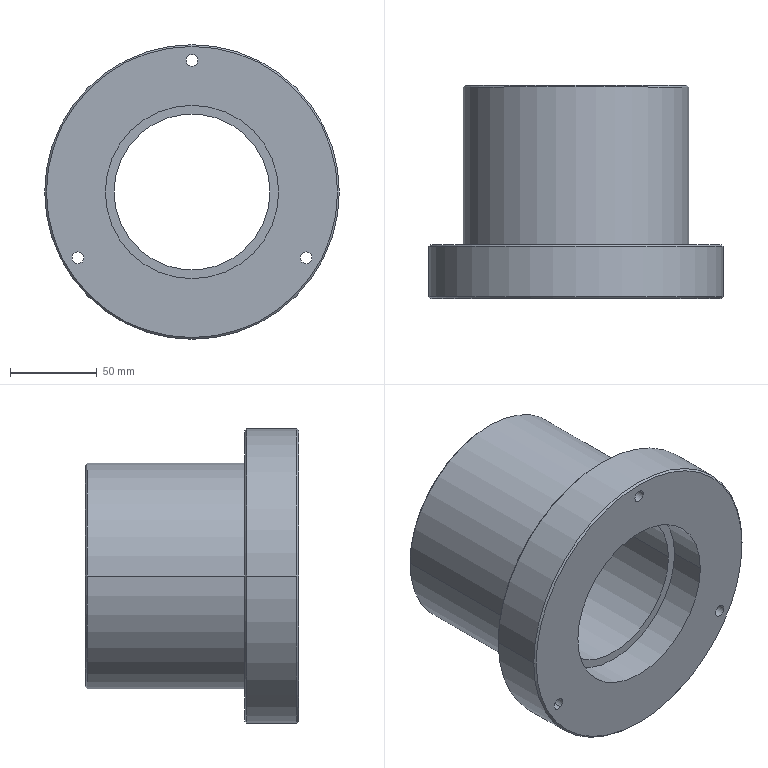Part | Creo | features CUT 9, CURVE 3, DATUM PLANE 3, PATTERN 2, CHAMFER 1, COORDINATE SYSTEM 1, PROTRUSION 1 | 1 solid | 45 faces | box 170 x 123 x 170 mm | volume 1070744 mm3 | cylinder 28 | plane 11 | cone 6 | commonest cylinder face diameters 5 x12 6.8 x6 100 x4 90 x2 130 x2 170 x2
STEP:
#1=CARTESIAN_POINT('',(0.,0.,0.));
#2=DIRECTION('',(0.,0.,1.));
#3=DIRECTION('',(1.,0.,0.));
#4=AXIS2_PLACEMENT_3D('',#1,#2,#3);
#5=CARTESIAN_POINT('',(50.,21.,0.));
#6=VERTEX_POINT('',#5);
#7=CARTESIAN_POINT('',(-50.,21.,0.));
#8=VERTEX_POINT('',#7);
#9=CARTESIAN_POINT('',(0.,21.,0.));
#10=DIRECTION('',(0.,-1.,0.));
#11=DIRECTION('',(1.,0.,0.));
#12=AXIS2_PLACEMENT_3D('',#9,#10,#11);
#13=CIRCLE('',#12,50.);
#14=EDGE_CURVE('',#6,#8,#13,.T.);
#15=ORIENTED_EDGE('',*,*,#14,.F.);
#16=CARTESIAN_POINT('',(0.,21.,0.));
#17=DIRECTION('',(0.,1.,0.));
#18=DIRECTION('',(1.,0.,0.));
#19=AXIS2_PLACEMENT_3D('',#16,#17,#18);
#20=CIRCLE('',#19,50.);
#21=EDGE_CURVE('',#6,#8,#20,.T.);
#22=ORIENTED_EDGE('',*,*,#21,.T.);
#23=EDGE_LOOP('',(#15,#22));
#24=FACE_OUTER_BOUND('',#23,.F.);
#25=CARTESIAN_POINT('',(45.,21.,0.));
#26=VERTEX_POINT('',#25);
#27=CARTESIAN_POINT('',(-45.,21.,0.));
#28=VERTEX_POINT('',#27);
#29=CARTESIAN_POINT('',(0.,21.,0.));
#30=DIRECTION('',(0.,1.,0.));
#31=DIRECTION('',(1.,0.,0.));
#32=AXIS2_PLACEMENT_3D('',#29,#30,#31);
#33=CIRCLE('',#32,45.);
#34=EDGE_CURVE('',#26,#28,#33,.T.);
#35=ORIENTED_EDGE('',*,*,#34,.F.);
#36=CARTESIAN_POINT('',(0.,21.,0.));
#37=DIRECTION('',(0.,-1.,0.));
#38=DIRECTION('',(1.,0.,0.));
#39=AXIS2_PLACEMENT_3D('',#36,#37,#38);
#40=CIRCLE('',#39,45.);
#41=EDGE_CURVE('',#26,#28,#40,.T.);
#42=ORIENTED_EDGE('',*,*,#41,.T.);
#43=EDGE_LOOP('',(#35,#42));
#44=FACE_BOUND('',#43,.F.);
#45=CARTESIAN_POINT('',(0.,21.,0.));
#46=DIRECTION('',(0.,1.,0.));
#47=DIRECTION('',(1.,0.,0.));
#48=AXIS2_PLACEMENT_3D('',#45,#46,#47);
#49=PLANE('',#48);
#50=ADVANCED_FACE('',(#24,#44),#49,.F.);
#51=CARTESIAN_POINT('',(45.,100.,0.));
#52=VERTEX_POINT('',#51);
#53=CARTESIAN_POINT('',(45.,100.,0.));
#54=DIRECTION('',(0.,-1.,0.));
#55=VECTOR('',#54,79.);
#56=LINE('',#53,#55);
#57=EDGE_CURVE('',#52,#26,#56,.T.);
#58=ORIENTED_EDGE('',*,*,#57,.T.);
#59=ORIENTED_EDGE('',*,*,#34,.T.);
#60=CARTESIAN_POINT('',(-45.,100.,0.));
#61=VERTEX_POINT('',#60);
#62=CARTESIAN_POINT('',(-45.,100.,0.));
#63=DIRECTION('',(0.,-1.,0.));
#64=VECTOR('',#63,79.);
#65=LINE('',#62,#64);
#66=EDGE_CURVE('',#61,#28,#65,.T.);
#67=ORIENTED_EDGE('',*,*,#66,.F.);
#68=CARTESIAN_POINT('',(0.,100.,0.));
#69=DIRECTION('',(0.,1.,0.));
#70=DIRECTION('',(1.,0.,0.));
#71=AXIS2_PLACEMENT_3D('',#68,#69,#70);
#72=CIRCLE('',#71,45.);
#73=EDGE_CURVE('',#52,#61,#72,.T.);
#74=ORIENTED_EDGE('',*,*,#73,.F.);
#75=EDGE_LOOP('',(#58,#59,#67,#74));
#76=FACE_OUTER_BOUND('',#75,.F.);
#77=CARTESIAN_POINT('',(0.,0.,0.));
#78=DIRECTION('',(0.,1.,0.));
#79=DIRECTION('',(1.,0.,0.));
#80=AXIS2_PLACEMENT_3D('',#77,#78,#79);
#81=CYLINDRICAL_SURFACE('',#80,45.);
#82=ADVANCED_FACE('',(#76),#81,.F.);
#83=ORIENTED_EDGE('',*,*,#57,.F.);
#84=CARTESIAN_POINT('',(0.,100.,0.));
#85=DIRECTION('',(0.,-1.,0.));
#86=DIRECTION('',(1.,0.,0.));
#87=AXIS2_PLACEMENT_3D('',#84,#85,#86);
#88=CIRCLE('',#87,45.);
#89=EDGE_CURVE('',#52,#61,#88,.T.);
#90=ORIENTED_EDGE('',*,*,#89,.T.);
#91=ORIENTED_EDGE('',*,*,#66,.T.);
#92=ORIENTED_EDGE('',*,*,#41,.F.);
#93=EDGE_LOOP('',(#83,#90,#91,#92));
#94=FACE_OUTER_BOUND('',#93,.F.);
#95=CARTESIAN_POINT('',(0.,0.,0.));
#96=DIRECTION('',(0.,1.,0.));
#97=DIRECTION('',(1.,0.,0.));
#98=AXIS2_PLACEMENT_3D('',#95,#96,#97);
#99=CYLINDRICAL_SURFACE('',#98,45.);
#100=ADVANCED_FACE('',(#94),#99,.F.);
#101=CARTESIAN_POINT('',(50.,100.,0.));
#102=VERTEX_POINT('',#101);
#103=CARTESIAN_POINT('',(-50.,100.,0.));
#104=VERTEX_POINT('',#103);
#105=CARTESIAN_POINT('',(0.,100.,0.));
#106=DIRECTION('',(0.,1.,0.));
#107=DIRECTION('',(1.,0.,0.));
#108=AXIS2_PLACEMENT_3D('',#105,#106,#107);
#109=CIRCLE('',#108,50.);
#110=EDGE_CURVE('',#102,#104,#109,.T.);
#111=ORIENTED_EDGE('',*,*,#110,.F.);
#112=CARTESIAN_POINT('',(0.,100.,0.));
#113=DIRECTION('',(0.,-1.,0.));
#114=DIRECTION('',(1.,0.,0.));
#115=AXIS2_PLACEMENT_3D('',#112,#113,#114);
#116=CIRCLE('',#115,50.);
#117=EDGE_CURVE('',#102,#104,#116,.T.);
#118=ORIENTED_EDGE('',*,*,#117,.T.);
#119=EDGE_LOOP('',(#111,#118));
#120=FACE_OUTER_BOUND('',#119,.F.);
#121=ORIENTED_EDGE('',*,*,#89,.F.);
#122=ORIENTED_EDGE('',*,*,#73,.T.);
#123=EDGE_LOOP('',(#121,#122));
#124=FACE_BOUND('',#123,.F.);
#125=CARTESIAN_POINT('',(0.,100.,0.));
#126=DIRECTION('',(0.,1.,0.));
#127=DIRECTION('',(1.,0.,0.));
#128=AXIS2_PLACEMENT_3D('',#125,#126,#127);
#129=PLANE('',#128);
#130=ADVANCED_FACE('',(#120,#124),#129,.T.);
#131=CARTESIAN_POINT('',(50.,123.,0.));
#132=VERTEX_POINT('',#131);
#133=CARTESIAN_POINT('',(50.,123.,0.));
#134=DIRECTION('',(0.,-1.,0.));
#135=VECTOR('',#134,23.);
#136=LINE('',#133,#135);
#137=EDGE_CURVE('',#132,#102,#136,.T.);
#138=ORIENTED_EDGE('',*,*,#137,.T.);
#139=ORIENTED_EDGE('',*,*,#110,.T.);
#140=CARTESIAN_POINT('',(-50.,123.,0.));
#141=VERTEX_POINT('',#140);
#142=CARTESIAN_POINT('',(-50.,123.,0.));
#143=DIRECTION('',(0.,-1.,0.));
#144=VECTOR('',#143,23.);
#145=LINE('',#142,#144);
#146=EDGE_CURVE('',#141,#104,#145,.T.);
#147=ORIENTED_EDGE('',*,*,#146,.F.);
#148=CARTESIAN_POINT('',(0.,123.,0.));
#149=DIRECTION('',(0.,1.,0.));
#150=DIRECTION('',(1.,0.,0.));
#151=AXIS2_PLACEMENT_3D('',#148,#149,#150);
#152=CIRCLE('',#151,50.);
#153=EDGE_CURVE('',#132,#141,#152,.T.);
#154=ORIENTED_EDGE('',*,*,#153,.F.);
#155=EDGE_LOOP('',(#138,#139,#147,#154));
#156=FACE_OUTER_BOUND('',#155,.F.);
#157=CARTESIAN_POINT('',(0.,0.,0.));
#158=DIRECTION('',(0.,1.,0.));
#159=DIRECTION('',(1.,0.,0.));
#160=AXIS2_PLACEMENT_3D('',#157,#158,#159);
#161=CYLINDRICAL_SURFACE('',#160,50.);
#162=ADVANCED_FACE('',(#156),#161,.F.);
#163=ORIENTED_EDGE('',*,*,#137,.F.);
#164=CARTESIAN_POINT('',(0.,123.,0.));
#165=DIRECTION('',(0.,-1.,0.));
#166=DIRECTION('',(1.,0.,0.));
#167=AXIS2_PLACEMENT_3D('',#164,#165,#166);
#168=CIRCLE('',#167,50.);
#169=EDGE_CURVE('',#132,#141,#168,.T.);
#170=ORIENTED_EDGE('',*,*,#169,.T.);
#171=ORIENTED_EDGE('',*,*,#146,.T.);
#172=ORIENTED_EDGE('',*,*,#117,.F.);
#173=EDGE_LOOP('',(#163,#170,#171,#172));
#174=FACE_OUTER_BOUND('',#173,.F.);
#175=CARTESIAN_POINT('',(0.,0.,0.));
#176=DIRECTION('',(0.,1.,0.));
#177=DIRECTION('',(1.,0.,0.));
#178=AXIS2_PLACEMENT_3D('',#175,#176,#177);
#179=CYLINDRICAL_SURFACE('',#178,50.);
#180=ADVANCED_FACE('',(#174),#179,.F.);
#181=CARTESIAN_POINT('',(64.,123.,0.));
#182=VERTEX_POINT('',#181);
#183=CARTESIAN_POINT('',(-64.,123.,0.));
#184=VERTEX_POINT('',#183);
#185=CARTESIAN_POINT('',(0.,123.,0.));
#186=DIRECTION('',(0.,1.,0.));
#187=DIRECTION('',(1.,0.,0.));
#188=AXIS2_PLACEMENT_3D('',#185,#186,#187);
#189=CIRCLE('',#188,64.);
#190=EDGE_CURVE('',#182,#184,#189,.T.);
#191=ORIENTED_EDGE('',*,*,#190,.F.);
#192=CARTESIAN_POINT('',(0.,123.,0.));
#193=DIRECTION('',(0.,1.,0.));
#194=DIRECTION('',(-1.,0.,0.));
#195=AXIS2_PLACEMENT_3D('',#192,#193,#194);
#196=CIRCLE('',#195,64.);
#197=EDGE_CURVE('',#184,#182,#196,.T.);
#198=ORIENTED_EDGE('',*,*,#197,.F.);
#199=EDGE_LOOP('',(#191,#198));
#200=FACE_OUTER_BOUND('',#199,.F.);
#201=ORIENTED_EDGE('',*,*,#169,.F.);
#202=ORIENTED_EDGE('',*,*,#153,.T.);
#203=EDGE_LOOP('',(#201,#202));
#204=FACE_BOUND('',#203,.F.);
#205=CARTESIAN_POINT('',(2.5,123.,-56.));
#206=VERTEX_POINT('',#205);
#207=CARTESIAN_POINT('',(-2.5,123.,-56.));
#208=VERTEX_POINT('',#207);
#209=CARTESIAN_POINT('',(0.,123.,-56.));
#210=DIRECTION('',(0.,1.,0.));
#211=DIRECTION('',(1.,0.,0.));
#212=AXIS2_PLACEMENT_3D('',#209,#210,#211);
#213=CIRCLE('',#212,2.5);
#214=EDGE_CURVE('',#206,#208,#213,.T.);
#215=ORIENTED_EDGE('',*,*,#214,.T.);
#216=CARTESIAN_POINT('',(0.,123.,-56.));
#217=DIRECTION('',(0.,1.,0.));
#218=DIRECTION('',(-1.,0.,0.));
#219=AXIS2_PLACEMENT_3D('',#216,#217,#218);
#220=CIRCLE('',#219,2.5);
#221=EDGE_CURVE('',#208,#206,#220,.T.);
#222=ORIENTED_EDGE('',*,*,#221,.T.);
#223=EDGE_LOOP('',(#215,#222));
#224=FACE_BOUND('',#223,.F.);
#225=CARTESIAN_POINT('',(-47.247,123.,-30.165));
#226=VERTEX_POINT('',#225);
#227=CARTESIAN_POINT('',(-49.747,123.,-25.835));
#228=VERTEX_POINT('',#227);
#229=CARTESIAN_POINT('',(-48.497,123.,-28.));
#230=DIRECTION('',(0.,1.,0.));
#231=DIRECTION('',(0.5,0.,-0.866));
#232=AXIS2_PLACEMENT_3D('',#229,#230,#231);
#233=CIRCLE('',#232,2.5);
#234=EDGE_CURVE('',#226,#228,#233,.T.);
#235=ORIENTED_EDGE('',*,*,#234,.T.);
#236=CARTESIAN_POINT('',(-48.497,123.,-28.));
#237=DIRECTION('',(0.,1.,0.));
#238=DIRECTION('',(-0.5,0.,0.866));
#239=AXIS2_PLACEMENT_3D('',#236,#237,#238);
#240=CIRCLE('',#239,2.5);
#241=EDGE_CURVE('',#228,#226,#240,.T.);
#242=ORIENTED_EDGE('',*,*,#241,.T.);
#243=EDGE_LOOP('',(#235,#242));
#244=FACE_BOUND('',#243,.F.);
#245=CARTESIAN_POINT('',(-49.747,123.,25.835));
#246=VERTEX_POINT('',#245);
#247=CARTESIAN_POINT('',(-47.247,123.,30.165));
#248=VERTEX_POINT('',#247);
#249=CARTESIAN_POINT('',(-48.497,123.,28.));
#250=DIRECTION('',(0.,1.,0.));
#251=DIRECTION('',(-0.5,0.,-0.866));
#252=AXIS2_PLACEMENT_3D('',#249,#250,#251);
#253=CIRCLE('',#252,2.5);
#254=EDGE_CURVE('',#246,#248,#253,.T.);
#255=ORIENTED_EDGE('',*,*,#254,.T.);
#256=CARTESIAN_POINT('',(-48.497,123.,28.));
#257=DIRECTION('',(0.,1.,0.));
#258=DIRECTION('',(0.5,0.,0.866));
#259=AXIS2_PLACEMENT_3D('',#256,#257,#258);
#260=CIRCLE('',#259,2.5);
#261=EDGE_CURVE('',#248,#246,#260,.T.);
#262=ORIENTED_EDGE('',*,*,#261,.T.);
#263=EDGE_LOOP('',(#255,#262));
#264=FACE_BOUND('',#263,.F.);
#265=CARTESIAN_POINT('',(-2.5,123.,56.));
#266=VERTEX_POINT('',#265);
#267=CARTESIAN_POINT('',(2.5,123.,56.));
#268=VERTEX_POINT('',#267);
#269=CARTESIAN_POINT('',(0.,123.,56.));
#270=DIRECTION('',(0.,1.,0.));
#271=DIRECTION('',(-1.,0.,0.));
#272=AXIS2_PLACEMENT_3D('',#269,#270,#271);
#273=CIRCLE('',#272,2.5);
#274=EDGE_CURVE('',#266,#268,#273,.T.);
#275=ORIENTED_EDGE('',*,*,#274,.T.);
#276=CARTESIAN_POINT('',(0.,123.,56.));
#277=DIRECTION('',(0.,1.,0.));
#278=DIRECTION('',(1.,0.,0.));
#279=AXIS2_PLACEMENT_3D('',#276,#277,#278);
#280=CIRCLE('',#279,2.5);
#281=EDGE_CURVE('',#268,#266,#280,.T.);
#282=ORIENTED_EDGE('',*,*,#281,.T.);
#283=EDGE_LOOP('',(#275,#282));
#284=FACE_BOUND('',#283,.F.);
#285=CARTESIAN_POINT('',(47.247,123.,30.165));
#286=VERTEX_POINT('',#285);
#287=CARTESIAN_POINT('',(49.747,123.,25.835));
#288=VERTEX_POINT('',#287);
#289=CARTESIAN_POINT('',(48.497,123.,28.));
#290=DIRECTION('',(0.,1.,0.));
#291=DIRECTION('',(-0.5,0.,0.866));
#292=AXIS2_PLACEMENT_3D('',#289,#290,#291);
#293=CIRCLE('',#292,2.5);
#294=EDGE_CURVE('',#286,#288,#293,.T.);
#295=ORIENTED_EDGE('',*,*,#294,.T.);
#296=CARTESIAN_POINT('',(48.497,123.,28.));
#297=DIRECTION('',(0.,1.,0.));
#298=DIRECTION('',(0.5,0.,-0.866));
#299=AXIS2_PLACEMENT_3D('',#296,#297,#298);
#300=CIRCLE('',#299,2.5);
#301=EDGE_CURVE('',#288,#286,#300,.T.);
#302=ORIENTED_EDGE('',*,*,#301,.T.);
#303=EDGE_LOOP('',(#295,#302));
#304=FACE_BOUND('',#303,.F.);
#305=CARTESIAN_POINT('',(49.747,123.,-25.835));
#306=VERTEX_POINT('',#305);
#307=CARTESIAN_POINT('',(47.247,123.,-30.165));
#308=VERTEX_POINT('',#307);
#309=CARTESIAN_POINT('',(48.497,123.,-28.));
#310=DIRECTION('',(0.,1.,0.));
#311=DIRECTION('',(0.5,0.,0.866));
#312=AXIS2_PLACEMENT_3D('',#309,#310,#311);
#313=CIRCLE('',#312,2.5);
#314=EDGE_CURVE('',#306,#308,#313,.T.);
#315=ORIENTED_EDGE('',*,*,#314,.T.);
#316=CARTESIAN_POINT('',(48.497,123.,-28.));
#317=DIRECTION('',(0.,1.,0.));
#318=DIRECTION('',(-0.5,0.,-0.866));
#319=AXIS2_PLACEMENT_3D('',#316,#317,#318);
#320=CIRCLE('',#319,2.5);
#321=EDGE_CURVE('',#308,#306,#320,.T.);
#322=ORIENTED_EDGE('',*,*,#321,.T.);
#323=EDGE_LOOP('',(#315,#322));
#324=FACE_BOUND('',#323,.F.);
#325=CARTESIAN_POINT('',(0.,123.,0.));
#326=DIRECTION('',(0.,1.,0.));
#327=DIRECTION('',(1.,0.,0.));
#328=AXIS2_PLACEMENT_3D('',#325,#326,#327);
#329=PLANE('',#328);
#330=ADVANCED_FACE('',(#200,#204,#224,#244,#264,#284,#304,#324),#329,.T.);
#331=ORIENTED_EDGE('',*,*,#190,.T.);
#332=CARTESIAN_POINT('',(-65.,122.,0.));
#333=VERTEX_POINT('',#332);
#334=CARTESIAN_POINT('',(-64.,123.,0.000000019));
#335=DIRECTION('',(-0.7071,-0.7071,-0.000000003));
#336=VECTOR('',#335,1.414);
#337=LINE('',#334,#336);
#338=EDGE_CURVE('',#184,#333,#337,.T.);
#339=ORIENTED_EDGE('',*,*,#338,.T.);
#340=CARTESIAN_POINT('',(65.,122.,0.));
#341=VERTEX_POINT('',#340);
#342=CARTESIAN_POINT('',(0.,122.,0.));
#343=DIRECTION('',(0.,1.,0.));
#344=DIRECTION('',(1.,0.,0.));
#345=AXIS2_PLACEMENT_3D('',#342,#343,#344);
#346=CIRCLE('',#345,65.);
#347=EDGE_CURVE('',#341,#333,#346,.T.);
#348=ORIENTED_EDGE('',*,*,#347,.F.);
#349=CARTESIAN_POINT('',(64.,123.,-0.000000019));
#350=DIRECTION('',(0.7071,-0.7071,0.000000003));
#351=VECTOR('',#350,1.414);
#352=LINE('',#349,#351);
#353=EDGE_CURVE('',#182,#341,#352,.T.);
#354=ORIENTED_EDGE('',*,*,#353,.F.);
#355=EDGE_LOOP('',(#331,#339,#348,#354));
#356=FACE_OUTER_BOUND('',#355,.F.);
#357=CARTESIAN_POINT('',(0.,122.5,0.));
#358=DIRECTION('',(0.,-1.,0.));
#359=DIRECTION('',(0.,0.,-1.));
#360=AXIS2_PLACEMENT_3D('',#357,#358,#359);
#361=CONICAL_SURFACE('',#360,64.5,45.);
#362=ADVANCED_FACE('',(#356),#361,.T.);
#363=ORIENTED_EDGE('',*,*,#197,.T.);
#364=ORIENTED_EDGE('',*,*,#353,.T.);
#365=CARTESIAN_POINT('',(0.,122.,0.));
#366=DIRECTION('',(0.,1.,0.));
#367=DIRECTION('',(-1.,0.,0.));
#368=AXIS2_PLACEMENT_3D('',#365,#366,#367);
#369=CIRCLE('',#368,65.);
#370=EDGE_CURVE('',#333,#341,#369,.T.);
#371=ORIENTED_EDGE('',*,*,#370,.F.);
#372=ORIENTED_EDGE('',*,*,#338,.F.);
#373=EDGE_LOOP('',(#363,#364,#371,#372));
#374=FACE_OUTER_BOUND('',#373,.F.);
#375=CARTESIAN_POINT('',(0.,122.5,0.));
#376=DIRECTION('',(0.,-1.,0.));
#377=DIRECTION('',(0.,0.,-1.));
#378=AXIS2_PLACEMENT_3D('',#375,#376,#377);
#379=CONICAL_SURFACE('',#378,64.5,45.);
#380=ADVANCED_FACE('',(#374),#379,.T.);
#381=ORIENTED_EDGE('',*,*,#370,.T.);
#382=CARTESIAN_POINT('',(65.,31.,0.));
#383=VERTEX_POINT('',#382);
#384=CARTESIAN_POINT('',(65.,31.,0.));
#385=DIRECTION('',(0.,1.,0.));
#386=VECTOR('',#385,91.);
#387=LINE('',#384,#386);
#388=EDGE_CURVE('',#383,#341,#387,.T.);
#389=ORIENTED_EDGE('',*,*,#388,.F.);
#390=CARTESIAN_POINT('',(-65.,31.,0.));
#391=VERTEX_POINT('',#390);
#392=CARTESIAN_POINT('',(0.,31.,0.));
#393=DIRECTION('',(0.,-1.,0.));
#394=DIRECTION('',(1.,0.,0.));
#395=AXIS2_PLACEMENT_3D('',#392,#393,#394);
#396=CIRCLE('',#395,65.);
#397=EDGE_CURVE('',#383,#391,#396,.T.);
#398=ORIENTED_EDGE('',*,*,#397,.T.);
#399=CARTESIAN_POINT('',(-65.,31.,0.));
#400=DIRECTION('',(0.,1.,0.));
#401=VECTOR('',#400,91.);
#402=LINE('',#399,#401);
#403=EDGE_CURVE('',#391,#333,#402,.T.);
#404=ORIENTED_EDGE('',*,*,#403,.T.);
#405=EDGE_LOOP('',(#381,#389,#398,#404));
#406=FACE_OUTER_BOUND('',#405,.F.);
#407=CARTESIAN_POINT('',(0.,0.,0.));
#408=DIRECTION('',(0.,1.,0.));
#409=DIRECTION('',(1.,0.,0.));
#410=AXIS2_PLACEMENT_3D('',#407,#408,#409);
#411=CYLINDRICAL_SURFACE('',#410,65.);
#412=ADVANCED_FACE('',(#406),#411,.T.);
#413=ORIENTED_EDGE('',*,*,#347,.T.);
#414=ORIENTED_EDGE('',*,*,#403,.F.);
#415=CARTESIAN_POINT('',(0.,31.,0.));
#416=DIRECTION('',(0.,1.,0.));
#417=DIRECTION('',(1.,0.,0.));
#418=AXIS2_PLACEMENT_3D('',#415,#416,#417);
#419=CIRCLE('',#418,65.);
#420=EDGE_CURVE('',#383,#391,#419,.T.);
#421=ORIENTED_EDGE('',*,*,#420,.F.);
#422=ORIENTED_EDGE('',*,*,#388,.T.);
#423=EDGE_LOOP('',(#413,#414,#421,#422));
#424=FACE_OUTER_BOUND('',#423,.F.);
#425=CARTESIAN_POINT('',(0.,0.,0.));
#426=DIRECTION('',(0.,1.,0.));
#427=DIRECTION('',(1.,0.,0.));
#428=AXIS2_PLACEMENT_3D('',#425,#426,#427);
#429=CYLINDRICAL_SURFACE('',#428,65.);
#430=ADVANCED_FACE('',(#424),#429,.T.);
#431=CARTESIAN_POINT('',(84.,31.,0.));
#432=VERTEX_POINT('',#431);
#433=CARTESIAN_POINT('',(-84.,31.,0.));
#434=VERTEX_POINT('',#433);
#435=CARTESIAN_POINT('',(0.,31.,0.));
#436=DIRECTION('',(0.,1.,0.));
#437=DIRECTION('',(1.,0.,0.));
#438=AXIS2_PLACEMENT_3D('',#435,#436,#437);
#439=CIRCLE('',#438,84.);
#440=EDGE_CURVE('',#432,#434,#439,.T.);
#441=ORIENTED_EDGE('',*,*,#440,.F.);
#442=CARTESIAN_POINT('',(0.,31.,0.));
#443=DIRECTION('',(0.,1.,0.));
#444=DIRECTION('',(-1.,0.,0.));
#445=AXIS2_PLACEMENT_3D('',#442,#443,#444);
#446=CIRCLE('',#445,84.);
#447=EDGE_CURVE('',#434,#432,#446,.T.);
#448=ORIENTED_EDGE('',*,*,#447,.F.);
#449=EDGE_LOOP('',(#441,#448));
#450=FACE_OUTER_BOUND('',#449,.F.);
#451=CARTESIAN_POINT('',(3.4,31.,76.));
#452=VERTEX_POINT('',#451);
#453=CARTESIAN_POINT('',(-3.4,31.,76.));
#454=VERTEX_POINT('',#453);
#455=CARTESIAN_POINT('',(0.,31.,76.));
#456=DIRECTION('',(0.,-1.,0.));
#457=DIRECTION('',(1.,0.,0.));
#458=AXIS2_PLACEMENT_3D('',#455,#456,#457);
#459=CIRCLE('',#458,3.4);
#460=EDGE_CURVE('',#452,#454,#459,.T.);
#461=ORIENTED_EDGE('',*,*,#460,.F.);
#462=CARTESIAN_POINT('',(0.,31.,76.));
#463=DIRECTION('',(0.,-1.,0.));
#464=DIRECTION('',(-1.,0.,0.));
#465=AXIS2_PLACEMENT_3D('',#462,#463,#464);
#466=CIRCLE('',#465,3.4);
#467=EDGE_CURVE('',#454,#452,#466,.T.);
#468=ORIENTED_EDGE('',*,*,#467,.F.);
#469=EDGE_LOOP('',(#461,#468));
#470=FACE_BOUND('',#469,.F.);
#471=CARTESIAN_POINT('',(64.118,31.,-40.944));
#472=VERTEX_POINT('',#471);
#473=CARTESIAN_POINT('',(67.518,31.,-35.056));
#474=VERTEX_POINT('',#473);
#475=CARTESIAN_POINT('',(65.818,31.,-38.));
#476=DIRECTION('',(0.,-1.,0.));
#477=DIRECTION('',(-0.5,0.,-0.866));
#478=AXIS2_PLACEMENT_3D('',#475,#476,#477);
#479=CIRCLE('',#478,3.4);
#480=EDGE_CURVE('',#472,#474,#479,.T.);
#481=ORIENTED_EDGE('',*,*,#480,.F.);
#482=CARTESIAN_POINT('',(65.818,31.,-38.));
#483=DIRECTION('',(0.,-1.,0.));
#484=DIRECTION('',(0.5,0.,0.866));
#485=AXIS2_PLACEMENT_3D('',#482,#483,#484);
#486=CIRCLE('',#485,3.4);
#487=EDGE_CURVE('',#474,#472,#486,.T.);
#488=ORIENTED_EDGE('',*,*,#487,.F.);
#489=EDGE_LOOP('',(#481,#488));
#490=FACE_BOUND('',#489,.F.);
#491=CARTESIAN_POINT('',(-67.518,31.,-35.056));
#492=VERTEX_POINT('',#491);
#493=CARTESIAN_POINT('',(-64.118,31.,-40.944));
#494=VERTEX_POINT('',#493);
#495=CARTESIAN_POINT('',(-65.818,31.,-38.));
#496=DIRECTION('',(0.,-1.,0.));
#497=DIRECTION('',(-0.5,0.,0.866));
#498=AXIS2_PLACEMENT_3D('',#495,#496,#497);
#499=CIRCLE('',#498,3.4);
#500=EDGE_CURVE('',#492,#494,#499,.T.);
#501=ORIENTED_EDGE('',*,*,#500,.F.);
#502=CARTESIAN_POINT('',(-65.818,31.,-38.));
#503=DIRECTION('',(0.,-1.,0.));
#504=DIRECTION('',(0.5,0.,-0.866));
#505=AXIS2_PLACEMENT_3D('',#502,#503,#504);
#506=CIRCLE('',#505,3.4);
#507=EDGE_CURVE('',#494,#492,#506,.T.);
#508=ORIENTED_EDGE('',*,*,#507,.F.);
#509=EDGE_LOOP('',(#501,#508));
#510=FACE_BOUND('',#509,.F.);
#511=ORIENTED_EDGE('',*,*,#397,.F.);
#512=ORIENTED_EDGE('',*,*,#420,.T.);
#513=EDGE_LOOP('',(#511,#512));
#514=FACE_BOUND('',#513,.F.);
#515=CARTESIAN_POINT('',(0.,31.,0.));
#516=DIRECTION('',(0.,1.,0.));
#517=DIRECTION('',(1.,0.,0.));
#518=AXIS2_PLACEMENT_3D('',#515,#516,#517);
#519=PLANE('',#518);
#520=ADVANCED_FACE('',(#450,#470,#490,#510,#514),#519,.T.);
#521=CARTESIAN_POINT('',(3.4,0.,76.));
#522=VERTEX_POINT('',#521);
#523=CARTESIAN_POINT('',(-3.4,0.,76.));
#524=VERTEX_POINT('',#523);
#525=CARTESIAN_POINT('',(0.,0.,76.));
#526=DIRECTION('',(0.,-1.,0.));
#527=DIRECTION('',(1.,0.,0.));
#528=AXIS2_PLACEMENT_3D('',#525,#526,#527);
#529=CIRCLE('',#528,3.4);
#530=EDGE_CURVE('',#522,#524,#529,.T.);
#531=ORIENTED_EDGE('',*,*,#530,.F.);
#532=CARTESIAN_POINT('',(3.4,0.,76.));
#533=DIRECTION('',(0.,1.,0.));
#534=VECTOR('',#533,31.);
#535=LINE('',#532,#534);
#536=EDGE_CURVE('',#522,#452,#535,.T.);
#537=ORIENTED_EDGE('',*,*,#536,.T.);
#538=ORIENTED_EDGE('',*,*,#460,.T.);
#539=CARTESIAN_POINT('',(-3.4,0.,76.));
#540=DIRECTION('',(0.,1.,0.));
#541=VECTOR('',#540,31.);
#542=LINE('',#539,#541);
#543=EDGE_CURVE('',#524,#454,#542,.T.);
#544=ORIENTED_EDGE('',*,*,#543,.F.);
#545=EDGE_LOOP('',(#531,#537,#538,#544));
#546=FACE_OUTER_BOUND('',#545,.F.);
#547=CARTESIAN_POINT('',(0.,0.,76.));
#548=DIRECTION('',(0.,-1.,0.));
#549=DIRECTION('',(1.,0.,0.));
#550=AXIS2_PLACEMENT_3D('',#547,#548,#549);
#551=CYLINDRICAL_SURFACE('',#550,3.4);
#552=ADVANCED_FACE('',(#546),#551,.F.);
#553=CARTESIAN_POINT('',(84.,0.,0.));
#554=VERTEX_POINT('',#553);
#555=CARTESIAN_POINT('',(-84.,0.,0.));
#556=VERTEX_POINT('',#555);
#557=CARTESIAN_POINT('',(0.,0.,0.));
#558=DIRECTION('',(0.,1.,0.));
#559=DIRECTION('',(1.,0.,0.));
#560=AXIS2_PLACEMENT_3D('',#557,#558,#559);
#561=CIRCLE('',#560,84.);
#562=EDGE_CURVE('',#554,#556,#561,.T.);
#563=ORIENTED_EDGE('',*,*,#562,.T.);
#564=CARTESIAN_POINT('',(0.,0.,0.));
#565=DIRECTION('',(0.,1.,0.));
#566=DIRECTION('',(-1.,0.,0.));
#567=AXIS2_PLACEMENT_3D('',#564,#565,#566);
#568=CIRCLE('',#567,84.);
#569=EDGE_CURVE('',#556,#554,#568,.T.);
#570=ORIENTED_EDGE('',*,*,#569,.T.);
#571=EDGE_LOOP('',(#563,#570));
#572=FACE_OUTER_BOUND('',#571,.F.);
#573=ORIENTED_EDGE('',*,*,#530,.T.);
#574=CARTESIAN_POINT('',(0.,0.,76.));
#575=DIRECTION('',(0.,-1.,0.));
#576=DIRECTION('',(-1.,0.,0.));
#577=AXIS2_PLACEMENT_3D('',#574,#575,#576);
#578=CIRCLE('',#577,3.4);
#579=EDGE_CURVE('',#524,#522,#578,.T.);
#580=ORIENTED_EDGE('',*,*,#579,.T.);
#581=EDGE_LOOP('',(#573,#580));
#582=FACE_BOUND('',#581,.F.);
#583=CARTESIAN_POINT('',(64.118,0.,-40.944));
#584=VERTEX_POINT('',#583);
#585=CARTESIAN_POINT('',(67.518,0.,-35.056));
#586=VERTEX_POINT('',#585);
#587=CARTESIAN_POINT('',(65.818,0.,-38.));
#588=DIRECTION('',(0.,-1.,0.));
#589=DIRECTION('',(-0.5,0.,-0.866));
#590=AXIS2_PLACEMENT_3D('',#587,#588,#589);
#591=CIRCLE('',#590,3.4);
#592=EDGE_CURVE('',#584,#586,#591,.T.);
#593=ORIENTED_EDGE('',*,*,#592,.T.);
#594=CARTESIAN_POINT('',(65.818,0.,-38.));
#595=DIRECTION('',(0.,-1.,0.));
#596=DIRECTION('',(0.5,0.,0.866));
#597=AXIS2_PLACEMENT_3D('',#594,#595,#596);
#598=CIRCLE('',#597,3.4);
#599=EDGE_CURVE('',#586,#584,#598,.T.);
#600=ORIENTED_EDGE('',*,*,#599,.T.);
#601=EDGE_LOOP('',(#593,#600));
#602=FACE_BOUND('',#601,.F.);
#603=CARTESIAN_POINT('',(-67.518,0.,-35.056));
#604=VERTEX_POINT('',#603);
#605=CARTESIAN_POINT('',(-64.118,0.,-40.944));
#606=VERTEX_POINT('',#605);
#607=CARTESIAN_POINT('',(-65.818,0.,-38.));
#608=DIRECTION('',(0.,-1.,0.));
#609=DIRECTION('',(-0.5,0.,0.866));
#610=AXIS2_PLACEMENT_3D('',#607,#608,#609);
#611=CIRCLE('',#610,3.4);
#612=EDGE_CURVE('',#604,#606,#611,.T.);
#613=ORIENTED_EDGE('',*,*,#612,.T.);
#614=CARTESIAN_POINT('',(-65.818,0.,-38.));
#615=DIRECTION('',(0.,-1.,0.));
#616=DIRECTION('',(0.5,0.,-0.866));
#617=AXIS2_PLACEMENT_3D('',#614,#615,#616);
#618=CIRCLE('',#617,3.4);
#619=EDGE_CURVE('',#606,#604,#618,.T.);
#620=ORIENTED_EDGE('',*,*,#619,.T.);
#621=EDGE_LOOP('',(#613,#620));
#622=FACE_BOUND('',#621,.F.);
#623=CARTESIAN_POINT('',(50.,0.,0.));
#624=VERTEX_POINT('',#623);
#625=CARTESIAN_POINT('',(-50.,0.,0.));
#626=VERTEX_POINT('',#625);
#627=CARTESIAN_POINT('',(0.,0.,0.));
#628=DIRECTION('',(0.,1.,0.));
#629=DIRECTION('',(1.,0.,0.));
#630=AXIS2_PLACEMENT_3D('',#627,#628,#629);
#631=CIRCLE('',#630,50.);
#632=EDGE_CURVE('',#624,#626,#631,.T.);
#633=ORIENTED_EDGE('',*,*,#632,.F.);
#634=CARTESIAN_POINT('',(0.,0.,0.));
#635=DIRECTION('',(0.,-1.,0.));
#636=DIRECTION('',(1.,0.,0.));
#637=AXIS2_PLACEMENT_3D('',#634,#635,#636);
#638=CIRCLE('',#637,50.);
#639=EDGE_CURVE('',#624,#626,#638,.T.);
#640=ORIENTED_EDGE('',*,*,#639,.T.);
#641=EDGE_LOOP('',(#633,#640));
#642=FACE_BOUND('',#641,.F.);
#643=CARTESIAN_POINT('',(0.,0.,0.));
#644=DIRECTION('',(0.,1.,0.));
#645=DIRECTION('',(1.,0.,0.));
#646=AXIS2_PLACEMENT_3D('',#643,#644,#645);
#647=PLANE('',#646);
#648=ADVANCED_FACE('',(#572,#582,#602,#622,#642),#647,.F.);
#649=CARTESIAN_POINT('',(50.,21.,0.));
#650=DIRECTION('',(0.,-1.,0.));
#651=VECTOR('',#650,21.);
#652=LINE('',#649,#651);
#653=EDGE_CURVE('',#6,#624,#652,.T.);
#654=ORIENTED_EDGE('',*,*,#653,.T.);
#655=ORIENTED_EDGE('',*,*,#632,.T.);
#656=CARTESIAN_POINT('',(-50.,21.,0.));
#657=DIRECTION('',(0.,-1.,0.));
#658=VECTOR('',#657,21.);
#659=LINE('',#656,#658);
#660=EDGE_CURVE('',#8,#626,#659,.T.);
#661=ORIENTED_EDGE('',*,*,#660,.F.);
#662=ORIENTED_EDGE('',*,*,#21,.F.);
#663=EDGE_LOOP('',(#654,#655,#661,#662));
#664=FACE_OUTER_BOUND('',#663,.F.);
#665=CARTESIAN_POINT('',(0.,0.,0.));
#666=DIRECTION('',(0.,1.,0.));
#667=DIRECTION('',(1.,0.,0.));
#668=AXIS2_PLACEMENT_3D('',#665,#666,#667);
#669=CYLINDRICAL_SURFACE('',#668,50.);
#670=ADVANCED_FACE('',(#664),#669,.F.);
#671=ORIENTED_EDGE('',*,*,#653,.F.);
#672=ORIENTED_EDGE('',*,*,#14,.T.);
#673=ORIENTED_EDGE('',*,*,#660,.T.);
#674=ORIENTED_EDGE('',*,*,#639,.F.);
#675=EDGE_LOOP('',(#671,#672,#673,#674));
#676=FACE_OUTER_BOUND('',#675,.F.);
#677=CARTESIAN_POINT('',(0.,0.,0.));
#678=DIRECTION('',(0.,1.,0.));
#679=DIRECTION('',(1.,0.,0.));
#680=AXIS2_PLACEMENT_3D('',#677,#678,#679);
#681=CYLINDRICAL_SURFACE('',#680,50.);
#682=ADVANCED_FACE('',(#676),#681,.F.);
#683=ORIENTED_EDGE('',*,*,#579,.F.);
#684=ORIENTED_EDGE('',*,*,#543,.T.);
#685=ORIENTED_EDGE('',*,*,#467,.T.);
#686=ORIENTED_EDGE('',*,*,#536,.F.);
#687=EDGE_LOOP('',(#683,#684,#685,#686));
#688=FACE_OUTER_BOUND('',#687,.F.);
#689=CARTESIAN_POINT('',(0.,0.,76.));
#690=DIRECTION('',(0.,-1.,0.));
#691=DIRECTION('',(1.,0.,0.));
#692=AXIS2_PLACEMENT_3D('',#689,#690,#691);
#693=CYLINDRICAL_SURFACE('',#692,3.4);
#694=ADVANCED_FACE('',(#688),#693,.F.);
#695=ORIENTED_EDGE('',*,*,#592,.F.);
#696=CARTESIAN_POINT('',(64.118,0.,-40.944));
#697=DIRECTION('',(0.,1.,0.));
#698=VECTOR('',#697,31.);
#699=LINE('',#696,#698);
#700=EDGE_CURVE('',#584,#472,#699,.T.);
#701=ORIENTED_EDGE('',*,*,#700,.T.);
#702=ORIENTED_EDGE('',*,*,#480,.T.);
#703=CARTESIAN_POINT('',(67.518,0.,-35.056));
#704=DIRECTION('',(0.,1.,0.));
#705=VECTOR('',#704,31.);
#706=LINE('',#703,#705);
#707=EDGE_CURVE('',#586,#474,#706,.T.);
#708=ORIENTED_EDGE('',*,*,#707,.F.);
#709=EDGE_LOOP('',(#695,#701,#702,#708));
#710=FACE_OUTER_BOUND('',#709,.F.);
#711=CARTESIAN_POINT('',(65.818,0.,-38.));
#712=DIRECTION('',(0.,-1.,0.));
#713=DIRECTION('',(-0.5,0.,-0.866));
#714=AXIS2_PLACEMENT_3D('',#711,#712,#713);
#715=CYLINDRICAL_SURFACE('',#714,3.4);
#716=ADVANCED_FACE('',(#710),#715,.F.);
#717=ORIENTED_EDGE('',*,*,#599,.F.);
#718=ORIENTED_EDGE('',*,*,#707,.T.);
#719=ORIENTED_EDGE('',*,*,#487,.T.);
#720=ORIENTED_EDGE('',*,*,#700,.F.);
#721=EDGE_LOOP('',(#717,#718,#719,#720));
#722=FACE_OUTER_BOUND('',#721,.F.);
#723=CARTESIAN_POINT('',(65.818,0.,-38.));
#724=DIRECTION('',(0.,-1.,0.));
#725=DIRECTION('',(-0.5,0.,-0.866));
#726=AXIS2_PLACEMENT_3D('',#723,#724,#725);
#727=CYLINDRICAL_SURFACE('',#726,3.4);
#728=ADVANCED_FACE('',(#722),#727,.F.);
#729=ORIENTED_EDGE('',*,*,#612,.F.);
#730=CARTESIAN_POINT('',(-67.518,0.,-35.056));
#731=DIRECTION('',(0.,1.,0.));
#732=VECTOR('',#731,31.);
#733=LINE('',#730,#732);
#734=EDGE_CURVE('',#604,#492,#733,.T.);
#735=ORIENTED_EDGE('',*,*,#734,.T.);
#736=ORIENTED_EDGE('',*,*,#500,.T.);
#737=CARTESIAN_POINT('',(-64.118,0.,-40.944));
#738=DIRECTION('',(0.,1.,0.));
#739=VECTOR('',#738,31.);
#740=LINE('',#737,#739);
#741=EDGE_CURVE('',#606,#494,#740,.T.);
#742=ORIENTED_EDGE('',*,*,#741,.F.);
#743=EDGE_LOOP('',(#729,#735,#736,#742));
#744=FACE_OUTER_BOUND('',#743,.F.);
#745=CARTESIAN_POINT('',(-65.818,0.,-38.));
#746=DIRECTION('',(0.,-1.,0.));
#747=DIRECTION('',(-0.5,0.,0.866));
#748=AXIS2_PLACEMENT_3D('',#745,#746,#747);
#749=CYLINDRICAL_SURFACE('',#748,3.4);
#750=ADVANCED_FACE('',(#744),#749,.F.);
#751=ORIENTED_EDGE('',*,*,#619,.F.);
#752=ORIENTED_EDGE('',*,*,#741,.T.);
#753=ORIENTED_EDGE('',*,*,#507,.T.);
#754=ORIENTED_EDGE('',*,*,#734,.F.);
#755=EDGE_LOOP('',(#751,#752,#753,#754));
#756=FACE_OUTER_BOUND('',#755,.F.);
#757=CARTESIAN_POINT('',(-65.818,0.,-38.));
#758=DIRECTION('',(0.,-1.,0.));
#759=DIRECTION('',(-0.5,0.,0.866));
#760=AXIS2_PLACEMENT_3D('',#757,#758,#759);
#761=CYLINDRICAL_SURFACE('',#760,3.4);
#762=ADVANCED_FACE('',(#756),#761,.F.);
#763=CARTESIAN_POINT('',(85.,1.,0.));
#764=VERTEX_POINT('',#763);
#765=CARTESIAN_POINT('',(-85.,1.,0.));
#766=VERTEX_POINT('',#765);
#767=CARTESIAN_POINT('',(0.,1.,0.));
#768=DIRECTION('',(0.,1.,0.));
#769=DIRECTION('',(1.,0.,0.));
#770=AXIS2_PLACEMENT_3D('',#767,#768,#769);
#771=CIRCLE('',#770,85.);
#772=EDGE_CURVE('',#764,#766,#771,.T.);
#773=ORIENTED_EDGE('',*,*,#772,.T.);
#774=CARTESIAN_POINT('',(-85.,1.,-0.000000002));
#775=DIRECTION('',(0.7071,-0.7071,-0.000000001));
#776=VECTOR('',#775,1.414);
#777=LINE('',#774,#776);
#778=EDGE_CURVE('',#766,#556,#777,.T.);
#779=ORIENTED_EDGE('',*,*,#778,.T.);
#780=ORIENTED_EDGE('',*,*,#562,.F.);
#781=CARTESIAN_POINT('',(85.,1.,0.000000002));
#782=DIRECTION('',(-0.7071,-0.7071,0.000000001));
#783=VECTOR('',#782,1.414);
#784=LINE('',#781,#783);
#785=EDGE_CURVE('',#764,#554,#784,.T.);
#786=ORIENTED_EDGE('',*,*,#785,.F.);
#787=EDGE_LOOP('',(#773,#779,#780,#786));
#788=FACE_OUTER_BOUND('',#787,.F.);
#789=CARTESIAN_POINT('',(0.,0.5,0.));
#790=DIRECTION('',(0.,1.,0.));
#791=DIRECTION('',(0.,0.,-1.));
#792=AXIS2_PLACEMENT_3D('',#789,#790,#791);
#793=CONICAL_SURFACE('',#792,84.5,45.);
#794=ADVANCED_FACE('',(#788),#793,.T.);
#795=ORIENTED_EDGE('',*,*,#772,.F.);
#796=CARTESIAN_POINT('',(85.,30.,0.));
#797=VERTEX_POINT('',#796);
#798=CARTESIAN_POINT('',(85.,1.,0.000000002));
#799=DIRECTION('',(0.,1.,0.));
#800=VECTOR('',#799,29.);
#801=LINE('',#798,#800);
#802=EDGE_CURVE('',#764,#797,#801,.T.);
#803=ORIENTED_EDGE('',*,*,#802,.T.);
#804=CARTESIAN_POINT('',(-85.,30.,0.));
#805=VERTEX_POINT('',#804);
#806=CARTESIAN_POINT('',(0.,30.,0.));
#807=DIRECTION('',(0.,1.,0.));
#808=DIRECTION('',(1.,0.,0.));
#809=AXIS2_PLACEMENT_3D('',#806,#807,#808);
#810=CIRCLE('',#809,85.);
#811=EDGE_CURVE('',#797,#805,#810,.T.);
#812=ORIENTED_EDGE('',*,*,#811,.T.);
#813=CARTESIAN_POINT('',(-85.,1.,-0.000000002));
#814=DIRECTION('',(0.,1.,0.));
#815=VECTOR('',#814,29.);
#816=LINE('',#813,#815);
#817=EDGE_CURVE('',#766,#805,#816,.T.);
#818=ORIENTED_EDGE('',*,*,#817,.F.);
#819=EDGE_LOOP('',(#795,#803,#812,#818));
#820=FACE_OUTER_BOUND('',#819,.F.);
#821=CARTESIAN_POINT('',(0.,0.,0.));
#822=DIRECTION('',(0.,1.,0.));
#823=DIRECTION('',(1.,0.,0.));
#824=AXIS2_PLACEMENT_3D('',#821,#822,#823);
#825=CYLINDRICAL_SURFACE('',#824,85.);
#826=ADVANCED_FACE('',(#820),#825,.T.);
#827=CARTESIAN_POINT('',(0.,1.,0.));
#828=DIRECTION('',(0.,1.,0.));
#829=DIRECTION('',(-1.,0.,0.));
#830=AXIS2_PLACEMENT_3D('',#827,#828,#829);
#831=CIRCLE('',#830,85.);
#832=EDGE_CURVE('',#766,#764,#831,.T.);
#833=ORIENTED_EDGE('',*,*,#832,.F.);
#834=ORIENTED_EDGE('',*,*,#817,.T.);
#835=CARTESIAN_POINT('',(0.,30.,0.));
#836=DIRECTION('',(0.,1.,0.));
#837=DIRECTION('',(-1.,0.,0.));
#838=AXIS2_PLACEMENT_3D('',#835,#836,#837);
#839=CIRCLE('',#838,85.);
#840=EDGE_CURVE('',#805,#797,#839,.T.);
#841=ORIENTED_EDGE('',*,*,#840,.T.);
#842=ORIENTED_EDGE('',*,*,#802,.F.);
#843=EDGE_LOOP('',(#833,#834,#841,#842));
#844=FACE_OUTER_BOUND('',#843,.F.);
#845=CARTESIAN_POINT('',(0.,0.,0.));
#846=DIRECTION('',(0.,1.,0.));
#847=DIRECTION('',(1.,0.,0.));
#848=AXIS2_PLACEMENT_3D('',#845,#846,#847);
#849=CYLINDRICAL_SURFACE('',#848,85.);
#850=ADVANCED_FACE('',(#844),#849,.T.);
#851=ORIENTED_EDGE('',*,*,#832,.T.);
#852=ORIENTED_EDGE('',*,*,#785,.T.);
#853=ORIENTED_EDGE('',*,*,#569,.F.);
#854=ORIENTED_EDGE('',*,*,#778,.F.);
#855=EDGE_LOOP('',(#851,#852,#853,#854));
#856=FACE_OUTER_BOUND('',#855,.F.);
#857=CARTESIAN_POINT('',(0.,0.5,0.));
#858=DIRECTION('',(0.,1.,0.));
#859=DIRECTION('',(0.,0.,-1.));
#860=AXIS2_PLACEMENT_3D('',#857,#858,#859);
#861=CONICAL_SURFACE('',#860,84.5,45.);
#862=ADVANCED_FACE('',(#856),#861,.T.);
#863=ORIENTED_EDGE('',*,*,#447,.T.);
#864=CARTESIAN_POINT('',(84.,31.,-0.000000013));
#865=DIRECTION('',(0.7071,-0.7071,0.000000002));
#866=VECTOR('',#865,1.414);
#867=LINE('',#864,#866);
#868=EDGE_CURVE('',#432,#797,#867,.T.);
#869=ORIENTED_EDGE('',*,*,#868,.T.);
#870=ORIENTED_EDGE('',*,*,#840,.F.);
#871=CARTESIAN_POINT('',(-84.,31.,0.000000013));
#872=DIRECTION('',(-0.7071,-0.7071,-0.000000002));
#873=VECTOR('',#872,1.414);
#874=LINE('',#871,#873);
#875=EDGE_CURVE('',#434,#805,#874,.T.);
#876=ORIENTED_EDGE('',*,*,#875,.F.);
#877=EDGE_LOOP('',(#863,#869,#870,#876));
#878=FACE_OUTER_BOUND('',#877,.F.);
#879=CARTESIAN_POINT('',(0.,30.5,0.));
#880=DIRECTION('',(0.,-1.,0.));
#881=DIRECTION('',(0.,0.,-1.));
#882=AXIS2_PLACEMENT_3D('',#879,#880,#881);
#883=CONICAL_SURFACE('',#882,84.5,45.);
#884=ADVANCED_FACE('',(#878),#883,.T.);
#885=ORIENTED_EDGE('',*,*,#440,.T.);
#886=ORIENTED_EDGE('',*,*,#875,.T.);
#887=ORIENTED_EDGE('',*,*,#811,.F.);
#888=ORIENTED_EDGE('',*,*,#868,.F.);
#889=EDGE_LOOP('',(#885,#886,#887,#888));
#890=FACE_OUTER_BOUND('',#889,.F.);
#891=CARTESIAN_POINT('',(0.,30.5,0.));
#892=DIRECTION('',(0.,-1.,0.));
#893=DIRECTION('',(0.,0.,-1.));
#894=AXIS2_PLACEMENT_3D('',#891,#892,#893);
#895=CONICAL_SURFACE('',#894,84.5,45.);
#896=ADVANCED_FACE('',(#890),#895,.T.);
#897=ORIENTED_EDGE('',*,*,#214,.F.);
#898=CARTESIAN_POINT('',(2.5,108.,-56.));
#899=VERTEX_POINT('',#898);
#900=CARTESIAN_POINT('',(2.5,123.,-56.));
#901=DIRECTION('',(0.,-1.,0.));
#902=VECTOR('',#901,15.);
#903=LINE('',#900,#902);
#904=EDGE_CURVE('',#206,#899,#903,.T.);
#905=ORIENTED_EDGE('',*,*,#904,.T.);
#906=CARTESIAN_POINT('',(-2.5,108.,-56.));
#907=VERTEX_POINT('',#906);
#908=CARTESIAN_POINT('',(0.,108.,-56.));
#909=DIRECTION('',(0.,1.,0.));
#910=DIRECTION('',(1.,0.,0.));
#911=AXIS2_PLACEMENT_3D('',#908,#909,#910);
#912=CIRCLE('',#911,2.5);
#913=EDGE_CURVE('',#899,#907,#912,.T.);
#914=ORIENTED_EDGE('',*,*,#913,.T.);
#915=CARTESIAN_POINT('',(-2.5,123.,-56.));
#916=DIRECTION('',(0.,-1.,0.));
#917=VECTOR('',#916,15.);
#918=LINE('',#915,#917);
#919=EDGE_CURVE('',#208,#907,#918,.T.);
#920=ORIENTED_EDGE('',*,*,#919,.F.);
#921=EDGE_LOOP('',(#897,#905,#914,#920));
#922=FACE_OUTER_BOUND('',#921,.F.);
#923=CARTESIAN_POINT('',(0.,123.,-56.));
#924=DIRECTION('',(0.,1.,0.));
#925=DIRECTION('',(1.,0.,0.));
#926=AXIS2_PLACEMENT_3D('',#923,#924,#925);
#927=CYLINDRICAL_SURFACE('',#926,2.5);
#928=ADVANCED_FACE('',(#922),#927,.F.);
#929=ORIENTED_EDGE('',*,*,#221,.F.);
#930=ORIENTED_EDGE('',*,*,#919,.T.);
#931=CARTESIAN_POINT('',(0.,108.,-56.));
#932=DIRECTION('',(0.,1.,0.));
#933=DIRECTION('',(-1.,0.,0.));
#934=AXIS2_PLACEMENT_3D('',#931,#932,#933);
#935=CIRCLE('',#934,2.5);
#936=EDGE_CURVE('',#907,#899,#935,.T.);
#937=ORIENTED_EDGE('',*,*,#936,.T.);
#938=ORIENTED_EDGE('',*,*,#904,.F.);
#939=EDGE_LOOP('',(#929,#930,#937,#938));
#940=FACE_OUTER_BOUND('',#939,.F.);
#941=CARTESIAN_POINT('',(0.,123.,-56.));
#942=DIRECTION('',(0.,1.,0.));
#943=DIRECTION('',(1.,0.,0.));
#944=AXIS2_PLACEMENT_3D('',#941,#942,#943);
#945=CYLINDRICAL_SURFACE('',#944,2.5);
#946=ADVANCED_FACE('',(#940),#945,.F.);
#947=ORIENTED_EDGE('',*,*,#913,.F.);
#948=ORIENTED_EDGE('',*,*,#936,.F.);
#949=EDGE_LOOP('',(#947,#948));
#950=FACE_OUTER_BOUND('',#949,.F.);
#951=CARTESIAN_POINT('',(0.,108.,0.));
#952=DIRECTION('',(0.,1.,0.));
#953=DIRECTION('',(1.,0.,0.));
#954=AXIS2_PLACEMENT_3D('',#951,#952,#953);
#955=PLANE('',#954);
#956=ADVANCED_FACE('',(#950),#955,.T.);
#957=ORIENTED_EDGE('',*,*,#234,.F.);
#958=CARTESIAN_POINT('',(-47.247,108.,-30.165));
#959=VERTEX_POINT('',#958);
#960=CARTESIAN_POINT('',(-47.247,123.,-30.165));
#961=DIRECTION('',(0.,-1.,0.));
#962=VECTOR('',#961,15.);
#963=LINE('',#960,#962);
#964=EDGE_CURVE('',#226,#959,#963,.T.);
#965=ORIENTED_EDGE('',*,*,#964,.T.);
#966=CARTESIAN_POINT('',(-49.747,108.,-25.835));
#967=VERTEX_POINT('',#966);
#968=CARTESIAN_POINT('',(-48.497,108.,-28.));
#969=DIRECTION('',(0.,1.,0.));
#970=DIRECTION('',(0.5,0.,-0.866));
#971=AXIS2_PLACEMENT_3D('',#968,#969,#970);
#972=CIRCLE('',#971,2.5);
#973=EDGE_CURVE('',#959,#967,#972,.T.);
#974=ORIENTED_EDGE('',*,*,#973,.T.);
#975=CARTESIAN_POINT('',(-49.747,123.,-25.835));
#976=DIRECTION('',(0.,-1.,0.));
#977=VECTOR('',#976,15.);
#978=LINE('',#975,#977);
#979=EDGE_CURVE('',#228,#967,#978,.T.);
#980=ORIENTED_EDGE('',*,*,#979,.F.);
#981=EDGE_LOOP('',(#957,#965,#974,#980));
#982=FACE_OUTER_BOUND('',#981,.F.);
#983=CARTESIAN_POINT('',(-48.497,123.,-28.));
#984=DIRECTION('',(0.,1.,0.));
#985=DIRECTION('',(0.5,0.,-0.866));
#986=AXIS2_PLACEMENT_3D('',#983,#984,#985);
#987=CYLINDRICAL_SURFACE('',#986,2.5);
#988=ADVANCED_FACE('',(#982),#987,.F.);
#989=ORIENTED_EDGE('',*,*,#241,.F.);
#990=ORIENTED_EDGE('',*,*,#979,.T.);
#991=CARTESIAN_POINT('',(-48.497,108.,-28.));
#992=DIRECTION('',(0.,1.,0.));
#993=DIRECTION('',(-0.5,0.,0.866));
#994=AXIS2_PLACEMENT_3D('',#991,#992,#993);
#995=CIRCLE('',#994,2.5);
#996=EDGE_CURVE('',#967,#959,#995,.T.);
#997=ORIENTED_EDGE('',*,*,#996,.T.);
#998=ORIENTED_EDGE('',*,*,#964,.F.);
#999=EDGE_LOOP('',(#989,#990,#997,#998));
#1000=FACE_OUTER_BOUND('',#999,.F.);
#1001=CARTESIAN_POINT('',(-48.497,123.,-28.));
#1002=DIRECTION('',(0.,1.,0.));
#1003=DIRECTION('',(0.5,0.,-0.866));
#1004=AXIS2_PLACEMENT_3D('',#1001,#1002,#1003);
#1005=CYLINDRICAL_SURFACE('',#1004,2.5);
#1006=ADVANCED_FACE('',(#1000),#1005,.F.);
#1007=ORIENTED_EDGE('',*,*,#973,.F.);
#1008=ORIENTED_EDGE('',*,*,#996,.F.);
#1009=EDGE_LOOP('',(#1007,#1008));
#1010=FACE_OUTER_BOUND('',#1009,.F.);
#1011=CARTESIAN_POINT('',(0.,108.,0.));
#1012=DIRECTION('',(0.,1.,0.));
#1013=DIRECTION('',(0.5,0.,-0.866));
#1014=AXIS2_PLACEMENT_3D('',#1011,#1012,#1013);
#1015=PLANE('',#1014);
#1016=ADVANCED_FACE('',(#1010),#1015,.T.);
#1017=ORIENTED_EDGE('',*,*,#254,.F.);
#1018=CARTESIAN_POINT('',(-49.747,108.,25.835));
#1019=VERTEX_POINT('',#1018);
#1020=CARTESIAN_POINT('',(-49.747,123.,25.835));
#1021=DIRECTION('',(0.,-1.,0.));
#1022=VECTOR('',#1021,15.);
#1023=LINE('',#1020,#1022);
#1024=EDGE_CURVE('',#246,#1019,#1023,.T.);
#1025=ORIENTED_EDGE('',*,*,#1024,.T.);
#1026=CARTESIAN_POINT('',(-47.247,108.,30.165));
#1027=VERTEX_POINT('',#1026);
#1028=CARTESIAN_POINT('',(-48.497,108.,28.));
#1029=DIRECTION('',(0.,1.,0.));
#1030=DIRECTION('',(-0.5,0.,-0.866));
#1031=AXIS2_PLACEMENT_3D('',#1028,#1029,#1030);
#1032=CIRCLE('',#1031,2.5);
#1033=EDGE_CURVE('',#1019,#1027,#1032,.T.);
#1034=ORIENTED_EDGE('',*,*,#1033,.T.);
#1035=CARTESIAN_POINT('',(-47.247,123.,30.165));
#1036=DIRECTION('',(0.,-1.,0.));
#1037=VECTOR('',#1036,15.);
#1038=LINE('',#1035,#1037);
#1039=EDGE_CURVE('',#248,#1027,#1038,.T.);
#1040=ORIENTED_EDGE('',*,*,#1039,.F.);
#1041=EDGE_LOOP('',(#1017,#1025,#1034,#1040));
#1042=FACE_OUTER_BOUND('',#1041,.F.);
#1043=CARTESIAN_POINT('',(-48.497,123.,28.));
#1044=DIRECTION('',(0.,1.,0.));
#1045=DIRECTION('',(-0.5,0.,-0.866));
#1046=AXIS2_PLACEMENT_3D('',#1043,#1044,#1045);
#1047=CYLINDRICAL_SURFACE('',#1046,2.5);
#1048=ADVANCED_FACE('',(#1042),#1047,.F.);
#1049=ORIENTED_EDGE('',*,*,#261,.F.);
#1050=ORIENTED_EDGE('',*,*,#1039,.T.);
#1051=CARTESIAN_POINT('',(-48.497,108.,28.));
#1052=DIRECTION('',(0.,1.,0.));
#1053=DIRECTION('',(0.5,0.,0.866));
#1054=AXIS2_PLACEMENT_3D('',#1051,#1052,#1053);
#1055=CIRCLE('',#1054,2.5);
#1056=EDGE_CURVE('',#1027,#1019,#1055,.T.);
#1057=ORIENTED_EDGE('',*,*,#1056,.T.);
#1058=ORIENTED_EDGE('',*,*,#1024,.F.);
#1059=EDGE_LOOP('',(#1049,#1050,#1057,#1058));
#1060=FACE_OUTER_BOUND('',#1059,.F.);
#1061=CARTESIAN_POINT('',(-48.497,123.,28.));
#1062=DIRECTION('',(0.,1.,0.));
#1063=DIRECTION('',(-0.5,0.,-0.866));
#1064=AXIS2_PLACEMENT_3D('',#1061,#1062,#1063);
#1065=CYLINDRICAL_SURFACE('',#1064,2.5);
#1066=ADVANCED_FACE('',(#1060),#1065,.F.);
#1067=ORIENTED_EDGE('',*,*,#1033,.F.);
#1068=ORIENTED_EDGE('',*,*,#1056,.F.);
#1069=EDGE_LOOP('',(#1067,#1068));
#1070=FACE_OUTER_BOUND('',#1069,.F.);
#1071=CARTESIAN_POINT('',(0.,108.,0.));
#1072=DIRECTION('',(0.,1.,0.));
#1073=DIRECTION('',(-0.5,0.,-0.866));
#1074=AXIS2_PLACEMENT_3D('',#1071,#1072,#1073);
#1075=PLANE('',#1074);
#1076=ADVANCED_FACE('',(#1070),#1075,.T.);
#1077=ORIENTED_EDGE('',*,*,#274,.F.);
#1078=CARTESIAN_POINT('',(-2.5,108.,56.));
#1079=VERTEX_POINT('',#1078);
#1080=CARTESIAN_POINT('',(-2.5,123.,56.));
#1081=DIRECTION('',(0.,-1.,0.));
#1082=VECTOR('',#1081,15.);
#1083=LINE('',#1080,#1082);
#1084=EDGE_CURVE('',#266,#1079,#1083,.T.);
#1085=ORIENTED_EDGE('',*,*,#1084,.T.);
#1086=CARTESIAN_POINT('',(2.5,108.,56.));
#1087=VERTEX_POINT('',#1086);
#1088=CARTESIAN_POINT('',(0.,108.,56.));
#1089=DIRECTION('',(0.,1.,0.));
#1090=DIRECTION('',(-1.,0.,0.));
#1091=AXIS2_PLACEMENT_3D('',#1088,#1089,#1090);
#1092=CIRCLE('',#1091,2.5);
#1093=EDGE_CURVE('',#1079,#1087,#1092,.T.);
#1094=ORIENTED_EDGE('',*,*,#1093,.T.);
#1095=CARTESIAN_POINT('',(2.5,123.,56.));
#1096=DIRECTION('',(0.,-1.,0.));
#1097=VECTOR('',#1096,15.);
#1098=LINE('',#1095,#1097);
#1099=EDGE_CURVE('',#268,#1087,#1098,.T.);
#1100=ORIENTED_EDGE('',*,*,#1099,.F.);
#1101=EDGE_LOOP('',(#1077,#1085,#1094,#1100));
#1102=FACE_OUTER_BOUND('',#1101,.F.);
#1103=CARTESIAN_POINT('',(0.,123.,56.));
#1104=DIRECTION('',(0.,1.,0.));
#1105=DIRECTION('',(-1.,0.,0.));
#1106=AXIS2_PLACEMENT_3D('',#1103,#1104,#1105);
#1107=CYLINDRICAL_SURFACE('',#1106,2.5);
#1108=ADVANCED_FACE('',(#1102),#1107,.F.);
#1109=ORIENTED_EDGE('',*,*,#281,.F.);
#1110=ORIENTED_EDGE('',*,*,#1099,.T.);
#1111=CARTESIAN_POINT('',(0.,108.,56.));
#1112=DIRECTION('',(0.,1.,0.));
#1113=DIRECTION('',(1.,0.,0.));
#1114=AXIS2_PLACEMENT_3D('',#1111,#1112,#1113);
#1115=CIRCLE('',#1114,2.5);
#1116=EDGE_CURVE('',#1087,#1079,#1115,.T.);
#1117=ORIENTED_EDGE('',*,*,#1116,.T.);
#1118=ORIENTED_EDGE('',*,*,#1084,.F.);
#1119=EDGE_LOOP('',(#1109,#1110,#1117,#1118));
#1120=FACE_OUTER_BOUND('',#1119,.F.);
#1121=CARTESIAN_POINT('',(0.,123.,56.));
#1122=DIRECTION('',(0.,1.,0.));
#1123=DIRECTION('',(-1.,0.,0.));
#1124=AXIS2_PLACEMENT_3D('',#1121,#1122,#1123);
#1125=CYLINDRICAL_SURFACE('',#1124,2.5);
#1126=ADVANCED_FACE('',(#1120),#1125,.F.);
#1127=ORIENTED_EDGE('',*,*,#1093,.F.);
#1128=ORIENTED_EDGE('',*,*,#1116,.F.);
#1129=EDGE_LOOP('',(#1127,#1128));
#1130=FACE_OUTER_BOUND('',#1129,.F.);
#1131=CARTESIAN_POINT('',(0.,108.,0.));
#1132=DIRECTION('',(0.,1.,0.));
#1133=DIRECTION('',(-1.,0.,0.));
#1134=AXIS2_PLACEMENT_3D('',#1131,#1132,#1133);
#1135=PLANE('',#1134);
#1136=ADVANCED_FACE('',(#1130),#1135,.T.);
#1137=ORIENTED_EDGE('',*,*,#294,.F.);
#1138=CARTESIAN_POINT('',(47.247,108.,30.165));
#1139=VERTEX_POINT('',#1138);
#1140=CARTESIAN_POINT('',(47.247,123.,30.165));
#1141=DIRECTION('',(0.,-1.,0.));
#1142=VECTOR('',#1141,15.);
#1143=LINE('',#1140,#1142);
#1144=EDGE_CURVE('',#286,#1139,#1143,.T.);
#1145=ORIENTED_EDGE('',*,*,#1144,.T.);
#1146=CARTESIAN_POINT('',(49.747,108.,25.835));
#1147=VERTEX_POINT('',#1146);
#1148=CARTESIAN_POINT('',(48.497,108.,28.));
#1149=DIRECTION('',(0.,1.,0.));
#1150=DIRECTION('',(-0.5,0.,0.866));
#1151=AXIS2_PLACEMENT_3D('',#1148,#1149,#1150);
#1152=CIRCLE('',#1151,2.5);
#1153=EDGE_CURVE('',#1139,#1147,#1152,.T.);
#1154=ORIENTED_EDGE('',*,*,#1153,.T.);
#1155=CARTESIAN_POINT('',(49.747,123.,25.835));
#1156=DIRECTION('',(0.,-1.,0.));
#1157=VECTOR('',#1156,15.);
#1158=LINE('',#1155,#1157);
#1159=EDGE_CURVE('',#288,#1147,#1158,.T.);
#1160=ORIENTED_EDGE('',*,*,#1159,.F.);
#1161=EDGE_LOOP('',(#1137,#1145,#1154,#1160));
#1162=FACE_OUTER_BOUND('',#1161,.F.);
#1163=CARTESIAN_POINT('',(48.497,123.,28.));
#1164=DIRECTION('',(0.,1.,0.));
#1165=DIRECTION('',(-0.5,0.,0.866));
#1166=AXIS2_PLACEMENT_3D('',#1163,#1164,#1165);
#1167=CYLINDRICAL_SURFACE('',#1166,2.5);
#1168=ADVANCED_FACE('',(#1162),#1167,.F.);
#1169=ORIENTED_EDGE('',*,*,#301,.F.);
#1170=ORIENTED_EDGE('',*,*,#1159,.T.);
#1171=CARTESIAN_POINT('',(48.497,108.,28.));
#1172=DIRECTION('',(0.,1.,0.));
#1173=DIRECTION('',(0.5,0.,-0.866));
#1174=AXIS2_PLACEMENT_3D('',#1171,#1172,#1173);
#1175=CIRCLE('',#1174,2.5);
#1176=EDGE_CURVE('',#1147,#1139,#1175,.T.);
#1177=ORIENTED_EDGE('',*,*,#1176,.T.);
#1178=ORIENTED_EDGE('',*,*,#1144,.F.);
#1179=EDGE_LOOP('',(#1169,#1170,#1177,#1178));
#1180=FACE_OUTER_BOUND('',#1179,.F.);
#1181=CARTESIAN_POINT('',(48.497,123.,28.));
#1182=DIRECTION('',(0.,1.,0.));
#1183=DIRECTION('',(-0.5,0.,0.866));
#1184=AXIS2_PLACEMENT_3D('',#1181,#1182,#1183);
#1185=CYLINDRICAL_SURFACE('',#1184,2.5);
#1186=ADVANCED_FACE('',(#1180),#1185,.F.);
#1187=ORIENTED_EDGE('',*,*,#1153,.F.);
#1188=ORIENTED_EDGE('',*,*,#1176,.F.);
#1189=EDGE_LOOP('',(#1187,#1188));
#1190=FACE_OUTER_BOUND('',#1189,.F.);
#1191=CARTESIAN_POINT('',(0.,108.,0.));
#1192=DIRECTION('',(0.,1.,0.));
#1193=DIRECTION('',(-0.5,0.,0.866));
#1194=AXIS2_PLACEMENT_3D('',#1191,#1192,#1193);
#1195=PLANE('',#1194);
#1196=ADVANCED_FACE('',(#1190),#1195,.T.);
#1197=ORIENTED_EDGE('',*,*,#314,.F.);
#1198=CARTESIAN_POINT('',(49.747,108.,-25.835));
#1199=VERTEX_POINT('',#1198);
#1200=CARTESIAN_POINT('',(49.747,123.,-25.835));
#1201=DIRECTION('',(0.,-1.,0.));
#1202=VECTOR('',#1201,15.);
#1203=LINE('',#1200,#1202);
#1204=EDGE_CURVE('',#306,#1199,#1203,.T.);
#1205=ORIENTED_EDGE('',*,*,#1204,.T.);
#1206=CARTESIAN_POINT('',(47.247,108.,-30.165));
#1207=VERTEX_POINT('',#1206);
#1208=CARTESIAN_POINT('',(48.497,108.,-28.));
#1209=DIRECTION('',(0.,1.,0.));
#1210=DIRECTION('',(0.5,0.,0.866));
#1211=AXIS2_PLACEMENT_3D('',#1208,#1209,#1210);
#1212=CIRCLE('',#1211,2.5);
#1213=EDGE_CURVE('',#1199,#1207,#1212,.T.);
#1214=ORIENTED_EDGE('',*,*,#1213,.T.);
#1215=CARTESIAN_POINT('',(47.247,123.,-30.165));
#1216=DIRECTION('',(0.,-1.,0.));
#1217=VECTOR('',#1216,15.);
#1218=LINE('',#1215,#1217);
#1219=EDGE_CURVE('',#308,#1207,#1218,.T.);
#1220=ORIENTED_EDGE('',*,*,#1219,.F.);
#1221=EDGE_LOOP('',(#1197,#1205,#1214,#1220));
#1222=FACE_OUTER_BOUND('',#1221,.F.);
#1223=CARTESIAN_POINT('',(48.497,123.,-28.));
#1224=DIRECTION('',(0.,1.,0.));
#1225=DIRECTION('',(0.5,0.,0.866));
#1226=AXIS2_PLACEMENT_3D('',#1223,#1224,#1225);
#1227=CYLINDRICAL_SURFACE('',#1226,2.5);
#1228=ADVANCED_FACE('',(#1222),#1227,.F.);
#1229=ORIENTED_EDGE('',*,*,#321,.F.);
#1230=ORIENTED_EDGE('',*,*,#1219,.T.);
#1231=CARTESIAN_POINT('',(48.497,108.,-28.));
#1232=DIRECTION('',(0.,1.,0.));
#1233=DIRECTION('',(-0.5,0.,-0.866));
#1234=AXIS2_PLACEMENT_3D('',#1231,#1232,#1233);
#1235=CIRCLE('',#1234,2.5);
#1236=EDGE_CURVE('',#1207,#1199,#1235,.T.);
#1237=ORIENTED_EDGE('',*,*,#1236,.T.);
#1238=ORIENTED_EDGE('',*,*,#1204,.F.);
#1239=EDGE_LOOP('',(#1229,#1230,#1237,#1238));
#1240=FACE_OUTER_BOUND('',#1239,.F.);
#1241=CARTESIAN_POINT('',(48.497,123.,-28.));
#1242=DIRECTION('',(0.,1.,0.));
#1243=DIRECTION('',(0.5,0.,0.866));
#1244=AXIS2_PLACEMENT_3D('',#1241,#1242,#1243);
#1245=CYLINDRICAL_SURFACE('',#1244,2.5);
#1246=ADVANCED_FACE('',(#1240),#1245,.F.);
#1247=ORIENTED_EDGE('',*,*,#1213,.F.);
#1248=ORIENTED_EDGE('',*,*,#1236,.F.);
#1249=EDGE_LOOP('',(#1247,#1248));
#1250=FACE_OUTER_BOUND('',#1249,.F.);
#1251=CARTESIAN_POINT('',(0.,108.,0.));
#1252=DIRECTION('',(0.,1.,0.));
#1253=DIRECTION('',(0.5,0.,0.866));
#1254=AXIS2_PLACEMENT_3D('',#1251,#1252,#1253);
#1255=PLANE('',#1254);
#1256=ADVANCED_FACE('',(#1250),#1255,.T.);
#1257=CLOSED_SHELL('',(#50,#82,#100,#130,#162,#180,#330,#362,#380,#412,#430,#520,#552,#648,#670,#682,#694,#716,#728,#750,#762,#794,#826,#850,#862,#884,#896,#928,#946,#956,#988,#1006,#1016,#1048,#1066,#1076,#1108,#1126,#1136,#1168,#1186,#1196,#1228,#1246,#1256));
#1258=MANIFOLD_SOLID_BREP('',#1257);
#1259=(LENGTH_UNIT()NAMED_UNIT(*)SI_UNIT(.MILLI.,.METRE.));
#1260=UNCERTAINTY_MEASURE_WITH_UNIT(LENGTH_MEASURE(0.02701),#1259,'','');
#1261=(NAMED_UNIT(*)PLANE_ANGLE_UNIT()SI_UNIT($,.RADIAN.));
#1262=PLANE_ANGLE_MEASURE_WITH_UNIT(PLANE_ANGLE_MEASURE(0.01745),#1261);
#1263=(CONVERSION_BASED_UNIT('DEGREE',#1262)NAMED_UNIT(*)PLANE_ANGLE_UNIT());
#1264=(NAMED_UNIT(*)SI_UNIT($,.STERADIAN.)SOLID_ANGLE_UNIT());
#1265=(GEOMETRIC_REPRESENTATION_CONTEXT(3)GLOBAL_UNCERTAINTY_ASSIGNED_CONTEXT((#1260))GLOBAL_UNIT_ASSIGNED_CONTEXT((#1259,#1263,#1264))REPRESENTATION_CONTEXT('',''));
#1266=ADVANCED_BREP_SHAPE_REPRESENTATION('',(#4,#1258),#1265);